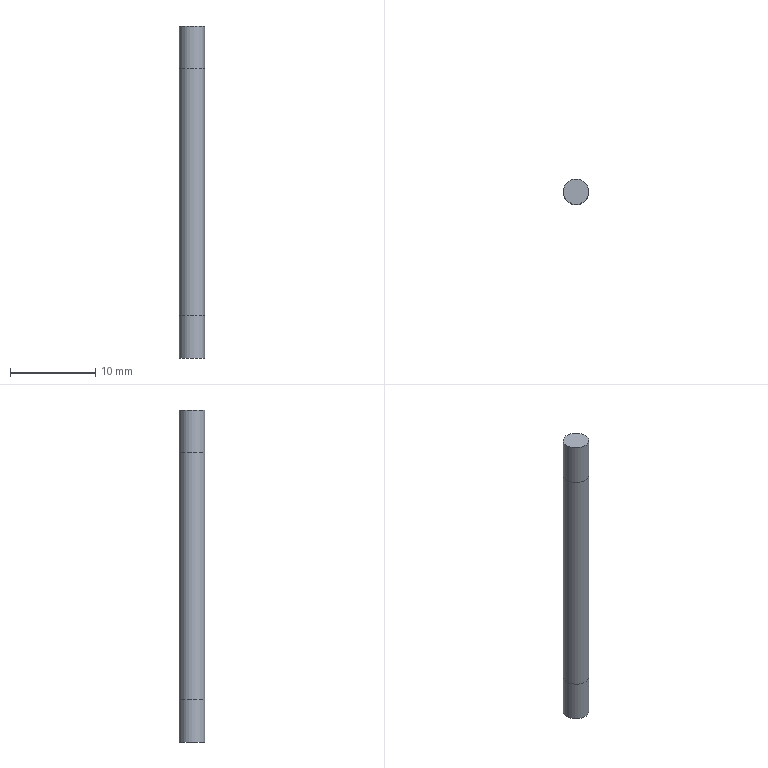Part | STEP file | 1-03.2 | 1 solid | 5 faces | box 3 x 3 x 39 mm | volume 275.675 mm3 | cylinder 3 | plane 2 | commonest cylinder face diameters 3 x3
STEP:
#1=CARTESIAN_POINT('',(0.,0.,0.));
#2=DIRECTION('',(0.,0.,1.));
#3=DIRECTION('',(1.,0.,0.));
#4=AXIS2_PLACEMENT_3D('',#1,#2,#3);
#5=CARTESIAN_POINT('',(1.5,0.,19.5));
#6=VERTEX_POINT('',#5);
#7=CARTESIAN_POINT('',(0.,0.,19.5));
#8=DIRECTION('',(0.,0.,1.));
#9=DIRECTION('',(1.,0.,0.));
#10=AXIS2_PLACEMENT_3D('',#7,#8,#9);
#11=CIRCLE('',#10,1.5);
#12=CARTESIAN_POINT('',(-0.4019,0.,19.5));
#13=DIRECTION('',(0.,0.,1.));
#14=DIRECTION('',(1.,0.,0.));
#15=AXIS2_PLACEMENT_3D('',#12,#13,#14);
#16=PLANE('',#15);
#17=CARTESIAN_POINT('',(0.4019,0.));
#18=DIRECTION('',(1.,0.));
#19=AXIS2_PLACEMENT_2D('',#17,#18);
#20=CIRCLE('',#19,1.5);
#21=(GEOMETRIC_REPRESENTATION_CONTEXT(2)PARAMETRIC_REPRESENTATION_CONTEXT()REPRESENTATION_CONTEXT('',''));
#22=DEFINITIONAL_REPRESENTATION('',(#20),#21);
#23=PCURVE('',#16,#22);
#24=CARTESIAN_POINT('',(0.,0.,19.5));
#25=DIRECTION('',(0.,0.,-1.));
#26=DIRECTION('',(1.,0.,0.));
#27=AXIS2_PLACEMENT_3D('',#24,#25,#26);
#28=CYLINDRICAL_SURFACE('',#27,1.5);
#29=CARTESIAN_POINT('',(6.283,0.));
#30=DIRECTION('',(-1.,0.));
#31=VECTOR('',#30,1.);
#32=LINE('',#29,#31);
#33=(GEOMETRIC_REPRESENTATION_CONTEXT(2)PARAMETRIC_REPRESENTATION_CONTEXT()REPRESENTATION_CONTEXT('',''));
#34=DEFINITIONAL_REPRESENTATION('',(#32),#33);
#35=PCURVE('',#28,#34);
#36=SURFACE_CURVE('',#11,(#23,#35),.PCURVE_S1.);
#37=EDGE_CURVE('',#6,#6,#36,.T.);
#38=ORIENTED_EDGE('',*,*,#37,.T.);
#39=EDGE_LOOP('',(#38));
#40=FACE_BOUND('',#39,.T.);
#41=ADVANCED_FACE('',(#40),#16,.T.);
#42=CARTESIAN_POINT('',(1.5,0.,-19.5));
#43=VERTEX_POINT('',#42);
#44=CARTESIAN_POINT('',(0.,0.,-19.5));
#45=DIRECTION('',(0.,0.,1.));
#46=DIRECTION('',(1.,0.,0.));
#47=AXIS2_PLACEMENT_3D('',#44,#45,#46);
#48=CIRCLE('',#47,1.5);
#49=CARTESIAN_POINT('',(-0.4019,0.,-19.5));
#50=DIRECTION('',(0.,0.,1.));
#51=DIRECTION('',(1.,0.,0.));
#52=AXIS2_PLACEMENT_3D('',#49,#50,#51);
#53=PLANE('',#52);
#54=CARTESIAN_POINT('',(0.4019,0.));
#55=DIRECTION('',(1.,0.));
#56=AXIS2_PLACEMENT_2D('',#54,#55);
#57=CIRCLE('',#56,1.5);
#58=(GEOMETRIC_REPRESENTATION_CONTEXT(2)PARAMETRIC_REPRESENTATION_CONTEXT()REPRESENTATION_CONTEXT('',''));
#59=DEFINITIONAL_REPRESENTATION('',(#57),#58);
#60=PCURVE('',#53,#59);
#61=CARTESIAN_POINT('',(0.,0.,-14.5));
#62=DIRECTION('',(0.,0.,-1.));
#63=DIRECTION('',(1.,0.,0.));
#64=AXIS2_PLACEMENT_3D('',#61,#62,#63);
#65=CYLINDRICAL_SURFACE('',#64,1.5);
#66=CARTESIAN_POINT('',(6.283,5.));
#67=DIRECTION('',(-1.,0.));
#68=VECTOR('',#67,1.);
#69=LINE('',#66,#68);
#70=(GEOMETRIC_REPRESENTATION_CONTEXT(2)PARAMETRIC_REPRESENTATION_CONTEXT()REPRESENTATION_CONTEXT('',''));
#71=DEFINITIONAL_REPRESENTATION('',(#69),#70);
#72=PCURVE('',#65,#71);
#73=SURFACE_CURVE('',#48,(#60,#72),.PCURVE_S1.);
#74=EDGE_CURVE('',#43,#43,#73,.T.);
#75=ORIENTED_EDGE('',*,*,#74,.T.);
#76=EDGE_LOOP('',(#75));
#77=FACE_BOUND('',#76,.F.);
#78=ADVANCED_FACE('',(#77),#53,.F.);
#79=CARTESIAN_POINT('',(1.5,0.,14.5));
#80=VERTEX_POINT('',#79);
#81=CARTESIAN_POINT('',(1.5,0.,19.5));
#82=DIRECTION('',(0.,0.,-1.));
#83=VECTOR('',#82,1.);
#84=LINE('',#81,#83);
#85=CARTESIAN_POINT('',(6.283,0.));
#86=DIRECTION('',(0.,1.));
#87=VECTOR('',#86,1.);
#88=LINE('',#85,#87);
#89=(GEOMETRIC_REPRESENTATION_CONTEXT(2)PARAMETRIC_REPRESENTATION_CONTEXT()REPRESENTATION_CONTEXT('',''));
#90=DEFINITIONAL_REPRESENTATION('',(#88),#89);
#91=PCURVE('',#28,#90);
#92=CARTESIAN_POINT('',(0.,0.));
#93=DIRECTION('',(0.,1.));
#94=VECTOR('',#93,1.);
#95=LINE('',#92,#94);
#96=(GEOMETRIC_REPRESENTATION_CONTEXT(2)PARAMETRIC_REPRESENTATION_CONTEXT()REPRESENTATION_CONTEXT('',''));
#97=DEFINITIONAL_REPRESENTATION('',(#95),#96);
#98=PCURVE('',#28,#97);
#99=SEAM_CURVE('',#84,(#91,#98),.PCURVE_S1.);
#100=EDGE_CURVE('',#6,#80,#99,.T.);
#101=ORIENTED_EDGE('',*,*,#100,.T.);
#102=CARTESIAN_POINT('',(0.,0.,14.5));
#103=DIRECTION('',(0.,0.,1.));
#104=DIRECTION('',(1.,0.,0.));
#105=AXIS2_PLACEMENT_3D('',#102,#103,#104);
#106=CIRCLE('',#105,1.5);
#107=CARTESIAN_POINT('',(6.283,5.));
#108=DIRECTION('',(-1.,0.));
#109=VECTOR('',#108,1.);
#110=LINE('',#107,#109);
#111=(GEOMETRIC_REPRESENTATION_CONTEXT(2)PARAMETRIC_REPRESENTATION_CONTEXT()REPRESENTATION_CONTEXT('',''));
#112=DEFINITIONAL_REPRESENTATION('',(#110),#111);
#113=PCURVE('',#28,#112);
#114=CARTESIAN_POINT('',(0.,0.,19.5));
#115=DIRECTION('',(0.,0.,-1.));
#116=DIRECTION('',(1.,0.,0.));
#117=AXIS2_PLACEMENT_3D('',#114,#115,#116);
#118=CYLINDRICAL_SURFACE('',#117,1.5);
#119=CARTESIAN_POINT('',(6.283,5.));
#120=DIRECTION('',(-1.,0.));
#121=VECTOR('',#120,1.);
#122=LINE('',#119,#121);
#123=(GEOMETRIC_REPRESENTATION_CONTEXT(2)PARAMETRIC_REPRESENTATION_CONTEXT()REPRESENTATION_CONTEXT('',''));
#124=DEFINITIONAL_REPRESENTATION('',(#122),#123);
#125=PCURVE('',#118,#124);
#126=SURFACE_CURVE('',#106,(#113,#125),.PCURVE_S1.);
#127=EDGE_CURVE('',#80,#80,#126,.T.);
#128=ORIENTED_EDGE('',*,*,#127,.T.);
#129=ORIENTED_EDGE('',*,*,#100,.F.);
#130=ORIENTED_EDGE('',*,*,#37,.F.);
#131=EDGE_LOOP('',(#101,#128,#129,#130));
#132=FACE_BOUND('',#131,.T.);
#133=ADVANCED_FACE('',(#132),#28,.T.);
#134=CARTESIAN_POINT('',(1.5,0.,-14.5));
#135=VERTEX_POINT('',#134);
#136=CARTESIAN_POINT('',(1.5,0.,14.5));
#137=DIRECTION('',(0.,0.,-1.));
#138=VECTOR('',#137,1.);
#139=LINE('',#136,#138);
#140=CARTESIAN_POINT('',(6.283,5.));
#141=DIRECTION('',(0.,1.));
#142=VECTOR('',#141,1.);
#143=LINE('',#140,#142);
#144=(GEOMETRIC_REPRESENTATION_CONTEXT(2)PARAMETRIC_REPRESENTATION_CONTEXT()REPRESENTATION_CONTEXT('',''));
#145=DEFINITIONAL_REPRESENTATION('',(#143),#144);
#146=PCURVE('',#118,#145);
#147=CARTESIAN_POINT('',(0.,5.));
#148=DIRECTION('',(0.,1.));
#149=VECTOR('',#148,1.);
#150=LINE('',#147,#149);
#151=(GEOMETRIC_REPRESENTATION_CONTEXT(2)PARAMETRIC_REPRESENTATION_CONTEXT()REPRESENTATION_CONTEXT('',''));
#152=DEFINITIONAL_REPRESENTATION('',(#150),#151);
#153=PCURVE('',#118,#152);
#154=SEAM_CURVE('',#139,(#146,#153),.PCURVE_S1.);
#155=EDGE_CURVE('',#80,#135,#154,.T.);
#156=ORIENTED_EDGE('',*,*,#155,.T.);
#157=CARTESIAN_POINT('',(0.,0.,-14.5));
#158=DIRECTION('',(0.,0.,1.));
#159=DIRECTION('',(1.,0.,0.));
#160=AXIS2_PLACEMENT_3D('',#157,#158,#159);
#161=CIRCLE('',#160,1.5);
#162=CARTESIAN_POINT('',(6.283,34.));
#163=DIRECTION('',(-1.,0.));
#164=VECTOR('',#163,1.);
#165=LINE('',#162,#164);
#166=(GEOMETRIC_REPRESENTATION_CONTEXT(2)PARAMETRIC_REPRESENTATION_CONTEXT()REPRESENTATION_CONTEXT('',''));
#167=DEFINITIONAL_REPRESENTATION('',(#165),#166);
#168=PCURVE('',#118,#167);
#169=CARTESIAN_POINT('',(6.283,0.));
#170=DIRECTION('',(-1.,0.));
#171=VECTOR('',#170,1.);
#172=LINE('',#169,#171);
#173=(GEOMETRIC_REPRESENTATION_CONTEXT(2)PARAMETRIC_REPRESENTATION_CONTEXT()REPRESENTATION_CONTEXT('',''));
#174=DEFINITIONAL_REPRESENTATION('',(#172),#173);
#175=PCURVE('',#65,#174);
#176=SURFACE_CURVE('',#161,(#168,#175),.PCURVE_S1.);
#177=EDGE_CURVE('',#135,#135,#176,.T.);
#178=ORIENTED_EDGE('',*,*,#177,.T.);
#179=ORIENTED_EDGE('',*,*,#155,.F.);
#180=ORIENTED_EDGE('',*,*,#127,.F.);
#181=EDGE_LOOP('',(#156,#178,#179,#180));
#182=FACE_BOUND('',#181,.T.);
#183=ADVANCED_FACE('',(#182),#118,.T.);
#184=CARTESIAN_POINT('',(1.5,0.,-14.5));
#185=DIRECTION('',(0.,0.,-1.));
#186=VECTOR('',#185,1.);
#187=LINE('',#184,#186);
#188=CARTESIAN_POINT('',(0.,0.));
#189=DIRECTION('',(0.,1.));
#190=VECTOR('',#189,1.);
#191=LINE('',#188,#190);
#192=(GEOMETRIC_REPRESENTATION_CONTEXT(2)PARAMETRIC_REPRESENTATION_CONTEXT()REPRESENTATION_CONTEXT('',''));
#193=DEFINITIONAL_REPRESENTATION('',(#191),#192);
#194=PCURVE('',#65,#193);
#195=CARTESIAN_POINT('',(6.283,0.));
#196=DIRECTION('',(0.,1.));
#197=VECTOR('',#196,1.);
#198=LINE('',#195,#197);
#199=(GEOMETRIC_REPRESENTATION_CONTEXT(2)PARAMETRIC_REPRESENTATION_CONTEXT()REPRESENTATION_CONTEXT('',''));
#200=DEFINITIONAL_REPRESENTATION('',(#198),#199);
#201=PCURVE('',#65,#200);
#202=SEAM_CURVE('',#187,(#194,#201),.PCURVE_S1.);
#203=EDGE_CURVE('',#135,#43,#202,.T.);
#204=ORIENTED_EDGE('',*,*,#203,.F.);
#205=ORIENTED_EDGE('',*,*,#177,.F.);
#206=ORIENTED_EDGE('',*,*,#203,.T.);
#207=ORIENTED_EDGE('',*,*,#74,.T.);
#208=EDGE_LOOP('',(#204,#205,#206,#207));
#209=FACE_BOUND('',#208,.T.);
#210=ADVANCED_FACE('',(#209),#65,.T.);
#211=CLOSED_SHELL('',(#41,#78,#133,#183,#210));
#212=MANIFOLD_SOLID_BREP('',#211);
#213=(LENGTH_UNIT()NAMED_UNIT(*)SI_UNIT(.MILLI.,.METRE.));
#214=UNCERTAINTY_MEASURE_WITH_UNIT(LENGTH_MEASURE(0.0000001),#213,'','');
#215=(NAMED_UNIT(*)PLANE_ANGLE_UNIT()SI_UNIT($,.RADIAN.));
#216=(NAMED_UNIT(*)SI_UNIT($,.STERADIAN.)SOLID_ANGLE_UNIT());
#217=(GEOMETRIC_REPRESENTATION_CONTEXT(3)GLOBAL_UNCERTAINTY_ASSIGNED_CONTEXT((#214))GLOBAL_UNIT_ASSIGNED_CONTEXT((#213,#215,#216))REPRESENTATION_CONTEXT('',''));
#218=ADVANCED_BREP_SHAPE_REPRESENTATION('',(#4,#212),#217);